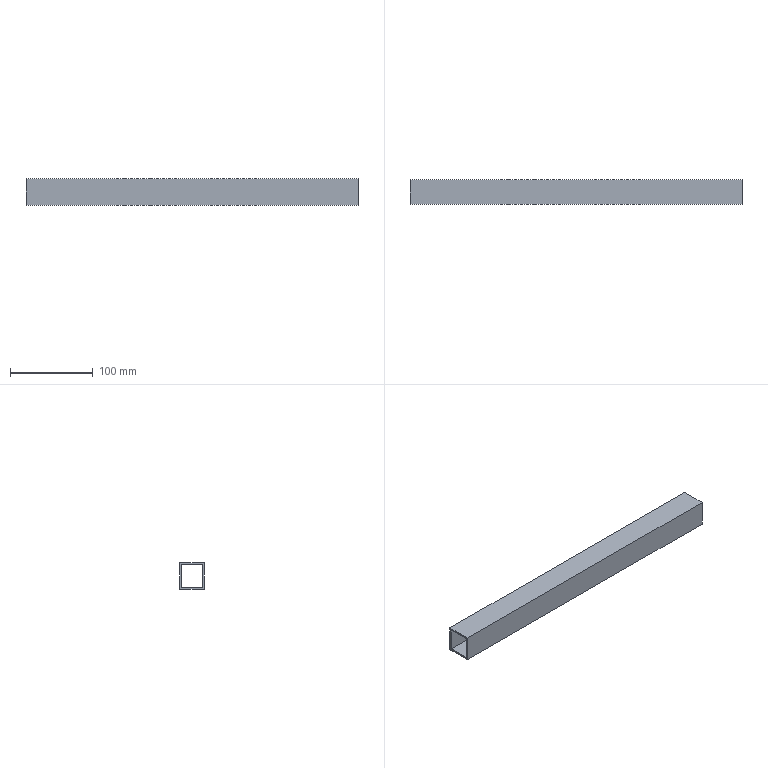Part | NX | features solid 2 | 1 solid | 10 faces | box 402 x 30 x 32 mm | volume 93264 mm3 | plane 10
STEP:
#1=CARTESIAN_POINT('',(43.,575.,-63.));
#2=VERTEX_POINT('',#1);
#3=CARTESIAN_POINT('',(43.,545.,-63.));
#4=VERTEX_POINT('',#3);
#5=CARTESIAN_POINT('',(43.,545.,-63.));
#6=DIRECTION('',(0.,1.,0.));
#7=VECTOR('',#6,1000.);
#8=LINE('',#5,#7);
#9=EDGE_CURVE('',#2,#4,#8,.F.);
#10=ORIENTED_EDGE('',*,*,#9,.F.);
#11=CARTESIAN_POINT('',(43.,575.,-95.));
#12=VERTEX_POINT('',#11);
#13=CARTESIAN_POINT('',(43.,575.,-63.));
#14=DIRECTION('',(0.,0.,1.));
#15=VECTOR('',#14,1000.);
#16=LINE('',#13,#15);
#17=EDGE_CURVE('',#2,#12,#16,.F.);
#18=ORIENTED_EDGE('',*,*,#17,.T.);
#19=CARTESIAN_POINT('',(43.,545.,-95.));
#20=VERTEX_POINT('',#19);
#21=CARTESIAN_POINT('',(43.,545.,-95.));
#22=DIRECTION('',(0.,-1.,0.));
#23=VECTOR('',#22,1000.);
#24=LINE('',#21,#23);
#25=EDGE_CURVE('',#12,#20,#24,.T.);
#26=ORIENTED_EDGE('',*,*,#25,.T.);
#27=CARTESIAN_POINT('',(43.,545.,-63.));
#28=DIRECTION('',(0.,0.,1.));
#29=VECTOR('',#28,1000.);
#30=LINE('',#27,#29);
#31=EDGE_CURVE('',#4,#20,#30,.F.);
#32=ORIENTED_EDGE('',*,*,#31,.F.);
#33=EDGE_LOOP('',(#10,#18,#26,#32));
#34=FACE_BOUND('',#33,.T.);
#35=CARTESIAN_POINT('',(43.,573.,-65.));
#36=VERTEX_POINT('',#35);
#37=CARTESIAN_POINT('',(43.,547.,-65.));
#38=VERTEX_POINT('',#37);
#39=CARTESIAN_POINT('',(43.,545.,-65.));
#40=DIRECTION('',(0.,1.,0.));
#41=VECTOR('',#40,1000.);
#42=LINE('',#39,#41);
#43=EDGE_CURVE('',#36,#38,#42,.F.);
#44=ORIENTED_EDGE('',*,*,#43,.T.);
#45=CARTESIAN_POINT('',(43.,547.,-93.));
#46=VERTEX_POINT('',#45);
#47=CARTESIAN_POINT('',(43.,547.,-63.));
#48=DIRECTION('',(0.,0.,1.));
#49=VECTOR('',#48,1000.);
#50=LINE('',#47,#49);
#51=EDGE_CURVE('',#38,#46,#50,.F.);
#52=ORIENTED_EDGE('',*,*,#51,.T.);
#53=CARTESIAN_POINT('',(43.,573.,-93.));
#54=VERTEX_POINT('',#53);
#55=CARTESIAN_POINT('',(43.,545.,-93.));
#56=DIRECTION('',(0.,-1.,0.));
#57=VECTOR('',#56,1000.);
#58=LINE('',#55,#57);
#59=EDGE_CURVE('',#54,#46,#58,.T.);
#60=ORIENTED_EDGE('',*,*,#59,.F.);
#61=CARTESIAN_POINT('',(43.,573.,-63.));
#62=DIRECTION('',(0.,0.,1.));
#63=VECTOR('',#62,1000.);
#64=LINE('',#61,#63);
#65=EDGE_CURVE('',#36,#54,#64,.F.);
#66=ORIENTED_EDGE('',*,*,#65,.F.);
#67=EDGE_LOOP('',(#44,#52,#60,#66));
#68=FACE_BOUND('',#67,.T.);
#69=CARTESIAN_POINT('',(43.,545.,-63.));
#70=DIRECTION('',(-1.,0.,0.));
#71=DIRECTION('',(0.,0.,-1.));
#72=AXIS2_PLACEMENT_3D('',#69,#70,#71);
#73=PLANE('',#72);
#74=ADVANCED_FACE('',(#34,#68),#73,.T.);
#75=CARTESIAN_POINT('',(445.,575.,-95.));
#76=VERTEX_POINT('',#75);
#77=CARTESIAN_POINT('',(445.,545.,-95.));
#78=VERTEX_POINT('',#77);
#79=CARTESIAN_POINT('',(445.,545.,-95.));
#80=DIRECTION('',(0.,-1.,0.));
#81=VECTOR('',#80,1000.);
#82=LINE('',#79,#81);
#83=EDGE_CURVE('',#76,#78,#82,.T.);
#84=ORIENTED_EDGE('',*,*,#83,.F.);
#85=CARTESIAN_POINT('',(445.,575.,-63.));
#86=VERTEX_POINT('',#85);
#87=CARTESIAN_POINT('',(445.,575.,-63.));
#88=DIRECTION('',(0.,0.,1.));
#89=VECTOR('',#88,1000.);
#90=LINE('',#87,#89);
#91=EDGE_CURVE('',#86,#76,#90,.F.);
#92=ORIENTED_EDGE('',*,*,#91,.F.);
#93=CARTESIAN_POINT('',(445.,545.,-63.));
#94=VERTEX_POINT('',#93);
#95=CARTESIAN_POINT('',(445.,378.,-63.));
#96=DIRECTION('',(0.,1.,0.));
#97=VECTOR('',#96,1000.);
#98=LINE('',#95,#97);
#99=EDGE_CURVE('',#86,#94,#98,.F.);
#100=ORIENTED_EDGE('',*,*,#99,.T.);
#101=CARTESIAN_POINT('',(445.,545.,-63.));
#102=DIRECTION('',(0.,0.,1.));
#103=VECTOR('',#102,1000.);
#104=LINE('',#101,#103);
#105=EDGE_CURVE('',#94,#78,#104,.F.);
#106=ORIENTED_EDGE('',*,*,#105,.T.);
#107=EDGE_LOOP('',(#84,#92,#100,#106));
#108=FACE_BOUND('',#107,.T.);
#109=CARTESIAN_POINT('',(445.,573.,-93.));
#110=VERTEX_POINT('',#109);
#111=CARTESIAN_POINT('',(445.,547.,-93.));
#112=VERTEX_POINT('',#111);
#113=CARTESIAN_POINT('',(445.,545.,-93.));
#114=DIRECTION('',(0.,-1.,0.));
#115=VECTOR('',#114,1000.);
#116=LINE('',#113,#115);
#117=EDGE_CURVE('',#110,#112,#116,.T.);
#118=ORIENTED_EDGE('',*,*,#117,.T.);
#119=CARTESIAN_POINT('',(445.,547.,-65.));
#120=VERTEX_POINT('',#119);
#121=CARTESIAN_POINT('',(445.,547.,-63.));
#122=DIRECTION('',(0.,0.,1.));
#123=VECTOR('',#122,1000.);
#124=LINE('',#121,#123);
#125=EDGE_CURVE('',#120,#112,#124,.F.);
#126=ORIENTED_EDGE('',*,*,#125,.F.);
#127=CARTESIAN_POINT('',(445.,573.,-65.));
#128=VERTEX_POINT('',#127);
#129=CARTESIAN_POINT('',(445.,378.,-65.));
#130=DIRECTION('',(0.,1.,0.));
#131=VECTOR('',#130,1000.);
#132=LINE('',#129,#131);
#133=EDGE_CURVE('',#128,#120,#132,.F.);
#134=ORIENTED_EDGE('',*,*,#133,.F.);
#135=CARTESIAN_POINT('',(445.,573.,-63.));
#136=DIRECTION('',(0.,0.,1.));
#137=VECTOR('',#136,1000.);
#138=LINE('',#135,#137);
#139=EDGE_CURVE('',#128,#110,#138,.F.);
#140=ORIENTED_EDGE('',*,*,#139,.T.);
#141=EDGE_LOOP('',(#118,#126,#134,#140));
#142=FACE_BOUND('',#141,.T.);
#143=CARTESIAN_POINT('',(445.,378.,-63.));
#144=DIRECTION('',(1.,0.,0.));
#145=DIRECTION('',(0.,0.,1.));
#146=AXIS2_PLACEMENT_3D('',#143,#144,#145);
#147=PLANE('',#146);
#148=ADVANCED_FACE('',(#108,#142),#147,.T.);
#149=ORIENTED_EDGE('',*,*,#25,.F.);
#150=CARTESIAN_POINT('',(53.,575.,-95.));
#151=DIRECTION('',(-1.,0.,0.));
#152=VECTOR('',#151,1000.);
#153=LINE('',#150,#152);
#154=EDGE_CURVE('',#12,#76,#153,.F.);
#155=ORIENTED_EDGE('',*,*,#154,.T.);
#156=ORIENTED_EDGE('',*,*,#83,.T.);
#157=CARTESIAN_POINT('',(53.,545.,-95.));
#158=DIRECTION('',(1.,0.,0.));
#159=VECTOR('',#158,1000.);
#160=LINE('',#157,#159);
#161=EDGE_CURVE('',#20,#78,#160,.T.);
#162=ORIENTED_EDGE('',*,*,#161,.F.);
#163=EDGE_LOOP('',(#149,#155,#156,#162));
#164=FACE_BOUND('',#163,.T.);
#165=CARTESIAN_POINT('',(53.,545.,-95.));
#166=DIRECTION('',(0.,0.,-1.));
#167=DIRECTION('',(1.,0.,0.));
#168=AXIS2_PLACEMENT_3D('',#165,#166,#167);
#169=PLANE('',#168);
#170=ADVANCED_FACE('',(#164),#169,.T.);
#171=CARTESIAN_POINT('',(53.,575.,-63.));
#172=DIRECTION('',(1.,0.,0.));
#173=VECTOR('',#172,1000.);
#174=LINE('',#171,#173);
#175=EDGE_CURVE('',#2,#86,#174,.T.);
#176=ORIENTED_EDGE('',*,*,#175,.F.);
#177=ORIENTED_EDGE('',*,*,#9,.T.);
#178=CARTESIAN_POINT('',(53.,545.,-63.));
#179=DIRECTION('',(1.,0.,0.));
#180=VECTOR('',#179,1000.);
#181=LINE('',#178,#180);
#182=EDGE_CURVE('',#4,#94,#181,.T.);
#183=ORIENTED_EDGE('',*,*,#182,.T.);
#184=ORIENTED_EDGE('',*,*,#99,.F.);
#185=EDGE_LOOP('',(#176,#177,#183,#184));
#186=FACE_BOUND('',#185,.T.);
#187=CARTESIAN_POINT('',(53.,545.,-63.));
#188=DIRECTION('',(0.,0.,-1.));
#189=DIRECTION('',(1.,0.,0.));
#190=AXIS2_PLACEMENT_3D('',#187,#188,#189);
#191=PLANE('',#190);
#192=ADVANCED_FACE('',(#186),#191,.F.);
#193=ORIENTED_EDGE('',*,*,#105,.F.);
#194=ORIENTED_EDGE('',*,*,#182,.F.);
#195=ORIENTED_EDGE('',*,*,#31,.T.);
#196=ORIENTED_EDGE('',*,*,#161,.T.);
#197=EDGE_LOOP('',(#193,#194,#195,#196));
#198=FACE_BOUND('',#197,.T.);
#199=CARTESIAN_POINT('',(53.,545.,-63.));
#200=DIRECTION('',(0.,1.,0.));
#201=DIRECTION('',(0.,0.,1.));
#202=AXIS2_PLACEMENT_3D('',#199,#200,#201);
#203=PLANE('',#202);
#204=ADVANCED_FACE('',(#198),#203,.F.);
#205=ORIENTED_EDGE('',*,*,#91,.T.);
#206=ORIENTED_EDGE('',*,*,#154,.F.);
#207=ORIENTED_EDGE('',*,*,#17,.F.);
#208=ORIENTED_EDGE('',*,*,#175,.T.);
#209=EDGE_LOOP('',(#205,#206,#207,#208));
#210=FACE_BOUND('',#209,.T.);
#211=CARTESIAN_POINT('',(53.,575.,-63.));
#212=DIRECTION('',(0.,1.,0.));
#213=DIRECTION('',(0.,0.,1.));
#214=AXIS2_PLACEMENT_3D('',#211,#212,#213);
#215=PLANE('',#214);
#216=ADVANCED_FACE('',(#210),#215,.T.);
#217=CARTESIAN_POINT('',(53.,547.,-93.));
#218=DIRECTION('',(-1.,0.,0.));
#219=VECTOR('',#218,1000.);
#220=LINE('',#217,#219);
#221=EDGE_CURVE('',#46,#112,#220,.F.);
#222=ORIENTED_EDGE('',*,*,#221,.T.);
#223=ORIENTED_EDGE('',*,*,#117,.F.);
#224=CARTESIAN_POINT('',(53.,573.,-93.));
#225=DIRECTION('',(-1.,0.,0.));
#226=VECTOR('',#225,1000.);
#227=LINE('',#224,#226);
#228=EDGE_CURVE('',#54,#110,#227,.F.);
#229=ORIENTED_EDGE('',*,*,#228,.F.);
#230=ORIENTED_EDGE('',*,*,#59,.T.);
#231=EDGE_LOOP('',(#222,#223,#229,#230));
#232=FACE_BOUND('',#231,.T.);
#233=CARTESIAN_POINT('',(53.,545.,-93.));
#234=DIRECTION('',(0.,0.,-1.));
#235=DIRECTION('',(1.,0.,0.));
#236=AXIS2_PLACEMENT_3D('',#233,#234,#235);
#237=PLANE('',#236);
#238=ADVANCED_FACE('',(#232),#237,.F.);
#239=CARTESIAN_POINT('',(53.,573.,-65.));
#240=DIRECTION('',(1.,0.,0.));
#241=VECTOR('',#240,1000.);
#242=LINE('',#239,#241);
#243=EDGE_CURVE('',#36,#128,#242,.T.);
#244=ORIENTED_EDGE('',*,*,#243,.T.);
#245=ORIENTED_EDGE('',*,*,#133,.T.);
#246=CARTESIAN_POINT('',(53.,547.,-65.));
#247=DIRECTION('',(1.,0.,0.));
#248=VECTOR('',#247,1000.);
#249=LINE('',#246,#248);
#250=EDGE_CURVE('',#38,#120,#249,.T.);
#251=ORIENTED_EDGE('',*,*,#250,.F.);
#252=ORIENTED_EDGE('',*,*,#43,.F.);
#253=EDGE_LOOP('',(#244,#245,#251,#252));
#254=FACE_BOUND('',#253,.T.);
#255=CARTESIAN_POINT('',(53.,545.,-65.));
#256=DIRECTION('',(0.,0.,-1.));
#257=DIRECTION('',(1.,0.,0.));
#258=AXIS2_PLACEMENT_3D('',#255,#256,#257);
#259=PLANE('',#258);
#260=ADVANCED_FACE('',(#254),#259,.T.);
#261=ORIENTED_EDGE('',*,*,#125,.T.);
#262=ORIENTED_EDGE('',*,*,#221,.F.);
#263=ORIENTED_EDGE('',*,*,#51,.F.);
#264=ORIENTED_EDGE('',*,*,#250,.T.);
#265=EDGE_LOOP('',(#261,#262,#263,#264));
#266=FACE_BOUND('',#265,.T.);
#267=CARTESIAN_POINT('',(53.,547.,-63.));
#268=DIRECTION('',(0.,1.,0.));
#269=DIRECTION('',(0.,0.,1.));
#270=AXIS2_PLACEMENT_3D('',#267,#268,#269);
#271=PLANE('',#270);
#272=ADVANCED_FACE('',(#266),#271,.T.);
#273=ORIENTED_EDGE('',*,*,#139,.F.);
#274=ORIENTED_EDGE('',*,*,#243,.F.);
#275=ORIENTED_EDGE('',*,*,#65,.T.);
#276=ORIENTED_EDGE('',*,*,#228,.T.);
#277=EDGE_LOOP('',(#273,#274,#275,#276));
#278=FACE_BOUND('',#277,.T.);
#279=CARTESIAN_POINT('',(53.,573.,-63.));
#280=DIRECTION('',(0.,1.,0.));
#281=DIRECTION('',(0.,0.,1.));
#282=AXIS2_PLACEMENT_3D('',#279,#280,#281);
#283=PLANE('',#282);
#284=ADVANCED_FACE('',(#278),#283,.F.);
#285=CLOSED_SHELL('',(#74,#148,#170,#192,#204,#216,#238,#260,#272,#284));
#286=MANIFOLD_SOLID_BREP('',#285);
#287=(LENGTH_UNIT()NAMED_UNIT(*)SI_UNIT(.MILLI.,.METRE.));
#288=UNCERTAINTY_MEASURE_WITH_UNIT(LENGTH_MEASURE(0.00001),#287,'','');
#289=(NAMED_UNIT(*)PLANE_ANGLE_UNIT()SI_UNIT($,.RADIAN.));
#290=(NAMED_UNIT(*)SI_UNIT($,.STERADIAN.)SOLID_ANGLE_UNIT());
#291=(GEOMETRIC_REPRESENTATION_CONTEXT(3)GLOBAL_UNCERTAINTY_ASSIGNED_CONTEXT((#288))GLOBAL_UNIT_ASSIGNED_CONTEXT((#287,#289,#290))REPRESENTATION_CONTEXT('',''));
#292=ADVANCED_BREP_SHAPE_REPRESENTATION('',(#286),#291);